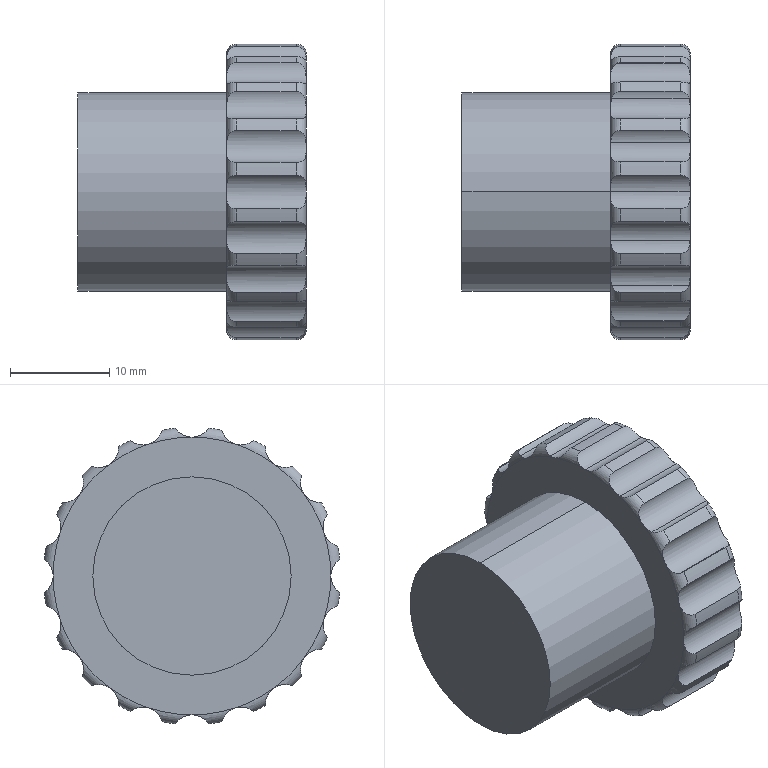Part | SolidWorks | features ICE 1, Revolution 1 | 1 solid | 92 faces | box 23 x 29.813 x 29.813 mm | volume 9978 mm3 | cylinder 49 | torus 40 | plane 3 | commonest cylinder face diameters 4 x27 30 x20 20 x2